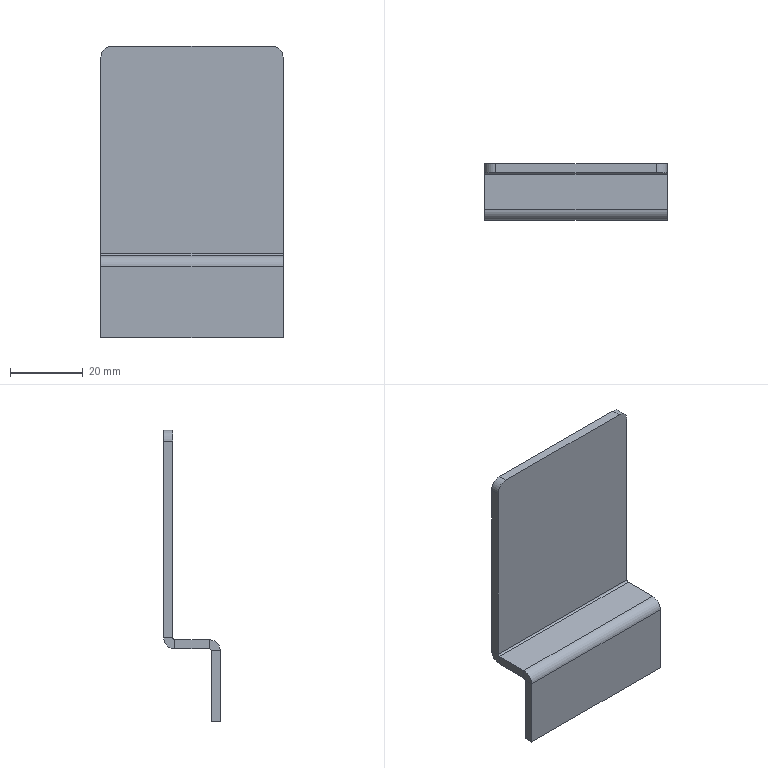Part | SolidWorks | features BaseBody 1 | 1 solid | 24 faces | box 50 x 15.5 x 80 mm | volume 11428 mm3 | plane 18 | cylinder 6 | commonest cylinder face diameters 6 x4 1 x2
STEP:
#1=CARTESIAN_POINT('',(-25.,-6.5,-22.5));
#2=VERTEX_POINT('',#1);
#3=CARTESIAN_POINT('',(25.,-6.5,-22.5));
#4=VERTEX_POINT('',#3);
#5=CARTESIAN_POINT('',(25.,-6.5,-22.5));
#6=DIRECTION('',(1.,0.,0.));
#7=VECTOR('',#6,1000.);
#8=LINE('',#5,#7);
#9=EDGE_CURVE('',#2,#4,#8,.T.);
#10=ORIENTED_EDGE('',*,*,#9,.T.);
#11=CARTESIAN_POINT('',(25.,-9.,-22.5));
#12=VERTEX_POINT('',#11);
#13=CARTESIAN_POINT('',(25.,-9.,-22.5));
#14=DIRECTION('',(0.,1.,0.));
#15=VECTOR('',#14,1000.);
#16=LINE('',#13,#15);
#17=EDGE_CURVE('',#12,#4,#16,.T.);
#18=ORIENTED_EDGE('',*,*,#17,.F.);
#19=CARTESIAN_POINT('',(-25.,-9.,-22.5));
#20=VERTEX_POINT('',#19);
#21=CARTESIAN_POINT('',(25.,-9.,-22.5));
#22=DIRECTION('',(1.,0.,0.));
#23=VECTOR('',#22,1000.);
#24=LINE('',#21,#23);
#25=EDGE_CURVE('',#20,#12,#24,.T.);
#26=ORIENTED_EDGE('',*,*,#25,.F.);
#27=CARTESIAN_POINT('',(-25.,-9.,-22.5));
#28=DIRECTION('',(0.,1.,0.));
#29=VECTOR('',#28,1000.);
#30=LINE('',#27,#29);
#31=EDGE_CURVE('',#20,#2,#30,.T.);
#32=ORIENTED_EDGE('',*,*,#31,.T.);
#33=EDGE_LOOP('',(#10,#18,#26,#32));
#34=FACE_OUTER_BOUND('',#33,.T.);
#35=CARTESIAN_POINT('',(25.,-9.,-22.5));
#36=DIRECTION('',(0.,0.,1.));
#37=DIRECTION('',(0.,-1.,0.));
#38=AXIS2_PLACEMENT_3D('',#35,#36,#37);
#39=PLANE('',#38);
#40=ADVANCED_FACE('',(#34),#39,.F.);
#41=CARTESIAN_POINT('',(-25.,-6.5,-3.));
#42=VERTEX_POINT('',#41);
#43=CARTESIAN_POINT('',(-25.,-6.5,-22.5));
#44=DIRECTION('',(0.,0.,-1.));
#45=VECTOR('',#44,1000.);
#46=LINE('',#43,#45);
#47=EDGE_CURVE('',#42,#2,#46,.T.);
#48=ORIENTED_EDGE('',*,*,#47,.F.);
#49=CARTESIAN_POINT('',(25.,-6.5,-3.));
#50=VERTEX_POINT('',#49);
#51=CARTESIAN_POINT('',(25.,-6.5,-3.));
#52=DIRECTION('',(-1.,0.,0.));
#53=VECTOR('',#52,1000.);
#54=LINE('',#51,#53);
#55=EDGE_CURVE('',#50,#42,#54,.T.);
#56=ORIENTED_EDGE('',*,*,#55,.F.);
#57=CARTESIAN_POINT('',(25.,-6.5,-2.5));
#58=DIRECTION('',(0.,0.,1.));
#59=VECTOR('',#58,1000.);
#60=LINE('',#57,#59);
#61=EDGE_CURVE('',#4,#50,#60,.T.);
#62=ORIENTED_EDGE('',*,*,#61,.F.);
#63=ORIENTED_EDGE('',*,*,#9,.F.);
#64=EDGE_LOOP('',(#48,#56,#62,#63));
#65=FACE_OUTER_BOUND('',#64,.T.);
#66=CARTESIAN_POINT('',(0.,-6.5,0.));
#67=DIRECTION('',(0.,1.,0.));
#68=DIRECTION('',(0.,0.,-1.));
#69=AXIS2_PLACEMENT_3D('',#66,#67,#68);
#70=PLANE('',#69);
#71=ADVANCED_FACE('',(#65),#70,.T.);
#72=CARTESIAN_POINT('',(-25.,-9.,-3.));
#73=VERTEX_POINT('',#72);
#74=CARTESIAN_POINT('',(25.,-9.,-3.));
#75=VERTEX_POINT('',#74);
#76=CARTESIAN_POINT('',(0.,-9.,-3.));
#77=DIRECTION('',(1.,0.,0.));
#78=VECTOR('',#77,1000.);
#79=LINE('',#76,#78);
#80=EDGE_CURVE('',#73,#75,#79,.T.);
#81=ORIENTED_EDGE('',*,*,#80,.F.);
#82=CARTESIAN_POINT('',(-25.,-9.,-22.5));
#83=DIRECTION('',(0.,0.,-1.));
#84=VECTOR('',#83,1000.);
#85=LINE('',#82,#84);
#86=EDGE_CURVE('',#73,#20,#85,.T.);
#87=ORIENTED_EDGE('',*,*,#86,.T.);
#88=ORIENTED_EDGE('',*,*,#25,.T.);
#89=CARTESIAN_POINT('',(25.,-9.,-2.5));
#90=DIRECTION('',(0.,0.,1.));
#91=VECTOR('',#90,1000.);
#92=LINE('',#89,#91);
#93=EDGE_CURVE('',#12,#75,#92,.T.);
#94=ORIENTED_EDGE('',*,*,#93,.T.);
#95=EDGE_LOOP('',(#81,#87,#88,#94));
#96=FACE_OUTER_BOUND('',#95,.T.);
#97=CARTESIAN_POINT('',(0.,-9.,0.));
#98=DIRECTION('',(0.,1.,0.));
#99=DIRECTION('',(0.,0.,-1.));
#100=AXIS2_PLACEMENT_3D('',#97,#98,#99);
#101=PLANE('',#100);
#102=ADVANCED_FACE('',(#96),#101,.F.);
#103=CARTESIAN_POINT('',(25.,-6.5,-3.));
#104=DIRECTION('',(0.,-1.,0.));
#105=VECTOR('',#104,1000.);
#106=LINE('',#103,#105);
#107=EDGE_CURVE('',#50,#75,#106,.T.);
#108=ORIENTED_EDGE('',*,*,#107,.T.);
#109=ORIENTED_EDGE('',*,*,#93,.F.);
#110=ORIENTED_EDGE('',*,*,#17,.T.);
#111=ORIENTED_EDGE('',*,*,#61,.T.);
#112=EDGE_LOOP('',(#108,#109,#110,#111));
#113=FACE_OUTER_BOUND('',#112,.T.);
#114=CARTESIAN_POINT('',(25.,-9.,-2.5));
#115=DIRECTION('',(-1.,0.,0.));
#116=DIRECTION('',(0.,1.,0.));
#117=AXIS2_PLACEMENT_3D('',#114,#115,#116);
#118=PLANE('',#117);
#119=ADVANCED_FACE('',(#113),#118,.F.);
#120=CARTESIAN_POINT('',(-25.,-6.5,-3.));
#121=DIRECTION('',(0.,-1.,0.));
#122=VECTOR('',#121,1000.);
#123=LINE('',#120,#122);
#124=EDGE_CURVE('',#42,#73,#123,.T.);
#125=ORIENTED_EDGE('',*,*,#124,.F.);
#126=ORIENTED_EDGE('',*,*,#47,.T.);
#127=ORIENTED_EDGE('',*,*,#31,.F.);
#128=ORIENTED_EDGE('',*,*,#86,.F.);
#129=EDGE_LOOP('',(#125,#126,#127,#128));
#130=FACE_OUTER_BOUND('',#129,.T.);
#131=CARTESIAN_POINT('',(-25.,-9.,-22.5));
#132=DIRECTION('',(1.,0.,0.));
#133=DIRECTION('',(0.,1.,0.));
#134=AXIS2_PLACEMENT_3D('',#131,#132,#133);
#135=PLANE('',#134);
#136=ADVANCED_FACE('',(#130),#135,.F.);
#137=CARTESIAN_POINT('',(-25.,-6.,-2.5));
#138=VERTEX_POINT('',#137);
#139=CARTESIAN_POINT('',(25.,-6.,-2.5));
#140=VERTEX_POINT('',#139);
#141=CARTESIAN_POINT('',(-25.,-6.,-2.5));
#142=DIRECTION('',(1.,0.,0.));
#143=VECTOR('',#142,1000.);
#144=LINE('',#141,#143);
#145=EDGE_CURVE('',#138,#140,#144,.T.);
#146=ORIENTED_EDGE('',*,*,#145,.T.);
#147=CARTESIAN_POINT('',(25.,-6.,-3.));
#148=DIRECTION('',(1.,0.,0.));
#149=DIRECTION('',(0.,0.,1.));
#150=AXIS2_PLACEMENT_3D('',#147,#148,#149);
#151=CIRCLE('',#150,0.5);
#152=EDGE_CURVE('',#140,#50,#151,.T.);
#153=ORIENTED_EDGE('',*,*,#152,.T.);
#154=ORIENTED_EDGE('',*,*,#55,.T.);
#155=CARTESIAN_POINT('',(-25.,-6.,-3.));
#156=DIRECTION('',(-1.,0.,0.));
#157=DIRECTION('',(0.,0.,1.));
#158=AXIS2_PLACEMENT_3D('',#155,#156,#157);
#159=CIRCLE('',#158,0.5);
#160=EDGE_CURVE('',#42,#138,#159,.T.);
#161=ORIENTED_EDGE('',*,*,#160,.T.);
#162=EDGE_LOOP('',(#146,#153,#154,#161));
#163=FACE_OUTER_BOUND('',#162,.T.);
#164=CARTESIAN_POINT('',(-25.,-6.,-3.));
#165=DIRECTION('',(-1.,0.,0.));
#166=DIRECTION('',(0.,-1.,0.));
#167=AXIS2_PLACEMENT_3D('',#164,#165,#166);
#168=CYLINDRICAL_SURFACE('',#167,0.5);
#169=ADVANCED_FACE('',(#163),#168,.F.);
#170=CARTESIAN_POINT('',(-25.,-6.,0.));
#171=VERTEX_POINT('',#170);
#172=CARTESIAN_POINT('',(25.,-6.,0.));
#173=VERTEX_POINT('',#172);
#174=CARTESIAN_POINT('',(-25.,-6.,0.));
#175=DIRECTION('',(1.,0.,0.));
#176=VECTOR('',#175,1000.);
#177=LINE('',#174,#176);
#178=EDGE_CURVE('',#171,#173,#177,.T.);
#179=ORIENTED_EDGE('',*,*,#178,.F.);
#180=CARTESIAN_POINT('',(-25.,-6.,-3.));
#181=DIRECTION('',(-1.,0.,0.));
#182=DIRECTION('',(0.,0.,1.));
#183=AXIS2_PLACEMENT_3D('',#180,#181,#182);
#184=CIRCLE('',#183,3.);
#185=EDGE_CURVE('',#73,#171,#184,.T.);
#186=ORIENTED_EDGE('',*,*,#185,.F.);
#187=ORIENTED_EDGE('',*,*,#80,.T.);
#188=CARTESIAN_POINT('',(25.,-6.,-3.));
#189=DIRECTION('',(1.,0.,0.));
#190=DIRECTION('',(0.,0.,1.));
#191=AXIS2_PLACEMENT_3D('',#188,#189,#190);
#192=CIRCLE('',#191,3.);
#193=EDGE_CURVE('',#173,#75,#192,.T.);
#194=ORIENTED_EDGE('',*,*,#193,.F.);
#195=EDGE_LOOP('',(#179,#186,#187,#194));
#196=FACE_OUTER_BOUND('',#195,.T.);
#197=CARTESIAN_POINT('',(-25.,-6.,-3.));
#198=DIRECTION('',(-1.,0.,0.));
#199=DIRECTION('',(0.,-1.,0.));
#200=AXIS2_PLACEMENT_3D('',#197,#198,#199);
#201=CYLINDRICAL_SURFACE('',#200,3.);
#202=ADVANCED_FACE('',(#196),#201,.T.);
#203=ORIENTED_EDGE('',*,*,#160,.F.);
#204=ORIENTED_EDGE('',*,*,#124,.T.);
#205=ORIENTED_EDGE('',*,*,#185,.T.);
#206=CARTESIAN_POINT('',(-25.,-6.,-2.5));
#207=DIRECTION('',(0.,0.,1.));
#208=VECTOR('',#207,1000.);
#209=LINE('',#206,#208);
#210=EDGE_CURVE('',#138,#171,#209,.T.);
#211=ORIENTED_EDGE('',*,*,#210,.F.);
#212=EDGE_LOOP('',(#203,#204,#205,#211));
#213=FACE_OUTER_BOUND('',#212,.T.);
#214=CARTESIAN_POINT('',(-25.,-6.,-3.));
#215=DIRECTION('',(1.,0.,0.));
#216=DIRECTION('',(0.,1.,0.));
#217=AXIS2_PLACEMENT_3D('',#214,#215,#216);
#218=PLANE('',#217);
#219=ADVANCED_FACE('',(#213),#218,.F.);
#220=ORIENTED_EDGE('',*,*,#107,.F.);
#221=ORIENTED_EDGE('',*,*,#152,.F.);
#222=CARTESIAN_POINT('',(25.,-6.,-2.5));
#223=DIRECTION('',(0.,0.,1.));
#224=VECTOR('',#223,1000.);
#225=LINE('',#222,#224);
#226=EDGE_CURVE('',#140,#173,#225,.T.);
#227=ORIENTED_EDGE('',*,*,#226,.T.);
#228=ORIENTED_EDGE('',*,*,#193,.T.);
#229=EDGE_LOOP('',(#220,#221,#227,#228));
#230=FACE_OUTER_BOUND('',#229,.T.);
#231=CARTESIAN_POINT('',(25.,-6.,-3.));
#232=DIRECTION('',(1.,0.,0.));
#233=DIRECTION('',(0.,1.,0.));
#234=AXIS2_PLACEMENT_3D('',#231,#232,#233);
#235=PLANE('',#234);
#236=ADVANCED_FACE('',(#230),#235,.T.);
#237=CARTESIAN_POINT('',(-25.,6.5,54.5));
#238=VERTEX_POINT('',#237);
#239=CARTESIAN_POINT('',(-22.,6.5,57.5));
#240=VERTEX_POINT('',#239);
#241=CARTESIAN_POINT('',(-22.,6.5,54.5));
#242=DIRECTION('',(0.,1.,0.));
#243=DIRECTION('',(0.,0.,-1.));
#244=AXIS2_PLACEMENT_3D('',#241,#242,#243);
#245=CIRCLE('',#244,3.);
#246=EDGE_CURVE('',#238,#240,#245,.T.);
#247=ORIENTED_EDGE('',*,*,#246,.F.);
#248=CARTESIAN_POINT('',(-25.,4.,54.5));
#249=VERTEX_POINT('',#248);
#250=CARTESIAN_POINT('',(-25.,6.5,54.5));
#251=DIRECTION('',(0.,1.,0.));
#252=VECTOR('',#251,1000.);
#253=LINE('',#250,#252);
#254=EDGE_CURVE('',#249,#238,#253,.T.);
#255=ORIENTED_EDGE('',*,*,#254,.F.);
#256=CARTESIAN_POINT('',(-22.,4.,57.5));
#257=VERTEX_POINT('',#256);
#258=CARTESIAN_POINT('',(-22.,4.,54.5));
#259=DIRECTION('',(0.,-1.,0.));
#260=DIRECTION('',(0.,0.,-1.));
#261=AXIS2_PLACEMENT_3D('',#258,#259,#260);
#262=CIRCLE('',#261,3.);
#263=EDGE_CURVE('',#257,#249,#262,.T.);
#264=ORIENTED_EDGE('',*,*,#263,.F.);
#265=CARTESIAN_POINT('',(-22.,6.5,57.5));
#266=DIRECTION('',(0.,-1.,0.));
#267=VECTOR('',#266,1000.);
#268=LINE('',#265,#267);
#269=EDGE_CURVE('',#240,#257,#268,.T.);
#270=ORIENTED_EDGE('',*,*,#269,.F.);
#271=EDGE_LOOP('',(#247,#255,#264,#270));
#272=FACE_OUTER_BOUND('',#271,.T.);
#273=CARTESIAN_POINT('',(-22.,6.5,54.5));
#274=DIRECTION('',(0.,-1.,0.));
#275=DIRECTION('',(0.,0.,-1.));
#276=AXIS2_PLACEMENT_3D('',#273,#274,#275);
#277=CYLINDRICAL_SURFACE('',#276,3.);
#278=ADVANCED_FACE('',(#272),#277,.T.);
#279=CARTESIAN_POINT('',(22.,6.5,57.5));
#280=VERTEX_POINT('',#279);
#281=CARTESIAN_POINT('',(25.,6.5,54.5));
#282=VERTEX_POINT('',#281);
#283=CARTESIAN_POINT('',(22.,6.5,54.5));
#284=DIRECTION('',(0.,1.,0.));
#285=DIRECTION('',(0.,0.,-1.));
#286=AXIS2_PLACEMENT_3D('',#283,#284,#285);
#287=CIRCLE('',#286,3.);
#288=EDGE_CURVE('',#280,#282,#287,.T.);
#289=ORIENTED_EDGE('',*,*,#288,.F.);
#290=CARTESIAN_POINT('',(22.,4.,57.5));
#291=VERTEX_POINT('',#290);
#292=CARTESIAN_POINT('',(22.,6.5,57.5));
#293=DIRECTION('',(0.,1.,0.));
#294=VECTOR('',#293,1000.);
#295=LINE('',#292,#294);
#296=EDGE_CURVE('',#291,#280,#295,.T.);
#297=ORIENTED_EDGE('',*,*,#296,.F.);
#298=CARTESIAN_POINT('',(25.,4.,54.5));
#299=VERTEX_POINT('',#298);
#300=CARTESIAN_POINT('',(22.,4.,54.5));
#301=DIRECTION('',(0.,-1.,0.));
#302=DIRECTION('',(0.,0.,-1.));
#303=AXIS2_PLACEMENT_3D('',#300,#301,#302);
#304=CIRCLE('',#303,3.);
#305=EDGE_CURVE('',#299,#291,#304,.T.);
#306=ORIENTED_EDGE('',*,*,#305,.F.);
#307=CARTESIAN_POINT('',(25.,6.5,54.5));
#308=DIRECTION('',(0.,-1.,0.));
#309=VECTOR('',#308,1000.);
#310=LINE('',#307,#309);
#311=EDGE_CURVE('',#282,#299,#310,.T.);
#312=ORIENTED_EDGE('',*,*,#311,.F.);
#313=EDGE_LOOP('',(#289,#297,#306,#312));
#314=FACE_OUTER_BOUND('',#313,.T.);
#315=CARTESIAN_POINT('',(22.,6.5,54.5));
#316=DIRECTION('',(0.,-1.,0.));
#317=DIRECTION('',(0.,0.,-1.));
#318=AXIS2_PLACEMENT_3D('',#315,#316,#317);
#319=CYLINDRICAL_SURFACE('',#318,3.);
#320=ADVANCED_FACE('',(#314),#319,.T.);
#321=CARTESIAN_POINT('',(25.,4.,57.5));
#322=DIRECTION('',(1.,0.,0.));
#323=VECTOR('',#322,1000.);
#324=LINE('',#321,#323);
#325=EDGE_CURVE('',#257,#291,#324,.T.);
#326=ORIENTED_EDGE('',*,*,#325,.T.);
#327=ORIENTED_EDGE('',*,*,#296,.T.);
#328=CARTESIAN_POINT('',(0.,6.5,57.5));
#329=DIRECTION('',(1.,0.,0.));
#330=VECTOR('',#329,1000.);
#331=LINE('',#328,#330);
#332=EDGE_CURVE('',#240,#280,#331,.T.);
#333=ORIENTED_EDGE('',*,*,#332,.F.);
#334=ORIENTED_EDGE('',*,*,#269,.T.);
#335=EDGE_LOOP('',(#326,#327,#333,#334));
#336=FACE_OUTER_BOUND('',#335,.T.);
#337=CARTESIAN_POINT('',(25.,6.5,57.5));
#338=DIRECTION('',(0.,0.,-1.));
#339=DIRECTION('',(0.,-1.,0.));
#340=AXIS2_PLACEMENT_3D('',#337,#338,#339);
#341=PLANE('',#340);
#342=ADVANCED_FACE('',(#336),#341,.F.);
#343=CARTESIAN_POINT('',(25.,4.,0.5));
#344=VERTEX_POINT('',#343);
#345=CARTESIAN_POINT('',(25.,4.,0.));
#346=DIRECTION('',(0.,0.,-1.));
#347=VECTOR('',#346,1000.);
#348=LINE('',#345,#347);
#349=EDGE_CURVE('',#299,#344,#348,.T.);
#350=ORIENTED_EDGE('',*,*,#349,.F.);
#351=ORIENTED_EDGE('',*,*,#305,.T.);
#352=ORIENTED_EDGE('',*,*,#325,.F.);
#353=ORIENTED_EDGE('',*,*,#263,.T.);
#354=CARTESIAN_POINT('',(-25.,4.,0.5));
#355=VERTEX_POINT('',#354);
#356=CARTESIAN_POINT('',(-25.,4.,57.5));
#357=DIRECTION('',(0.,0.,1.));
#358=VECTOR('',#357,1000.);
#359=LINE('',#356,#358);
#360=EDGE_CURVE('',#355,#249,#359,.T.);
#361=ORIENTED_EDGE('',*,*,#360,.F.);
#362=CARTESIAN_POINT('',(25.,4.,0.5));
#363=DIRECTION('',(-1.,0.,0.));
#364=VECTOR('',#363,1000.);
#365=LINE('',#362,#364);
#366=EDGE_CURVE('',#344,#355,#365,.T.);
#367=ORIENTED_EDGE('',*,*,#366,.F.);
#368=EDGE_LOOP('',(#350,#351,#352,#353,#361,#367));
#369=FACE_OUTER_BOUND('',#368,.T.);
#370=CARTESIAN_POINT('',(0.,4.,0.));
#371=DIRECTION('',(0.,-1.,0.));
#372=DIRECTION('',(-1.,0.,0.));
#373=AXIS2_PLACEMENT_3D('',#370,#371,#372);
#374=PLANE('',#373);
#375=ADVANCED_FACE('',(#369),#374,.T.);
#376=ORIENTED_EDGE('',*,*,#332,.T.);
#377=ORIENTED_EDGE('',*,*,#288,.T.);
#378=CARTESIAN_POINT('',(25.,6.5,0.5));
#379=VERTEX_POINT('',#378);
#380=CARTESIAN_POINT('',(25.,6.5,0.));
#381=DIRECTION('',(0.,0.,-1.));
#382=VECTOR('',#381,1000.);
#383=LINE('',#380,#382);
#384=EDGE_CURVE('',#282,#379,#383,.T.);
#385=ORIENTED_EDGE('',*,*,#384,.T.);
#386=CARTESIAN_POINT('',(-25.,6.5,0.5));
#387=VERTEX_POINT('',#386);
#388=CARTESIAN_POINT('',(25.,6.5,0.5));
#389=DIRECTION('',(1.,0.,0.));
#390=VECTOR('',#389,1000.);
#391=LINE('',#388,#390);
#392=EDGE_CURVE('',#387,#379,#391,.T.);
#393=ORIENTED_EDGE('',*,*,#392,.F.);
#394=CARTESIAN_POINT('',(-25.,6.5,0.));
#395=DIRECTION('',(0.,0.,1.));
#396=VECTOR('',#395,1000.);
#397=LINE('',#394,#396);
#398=EDGE_CURVE('',#387,#238,#397,.T.);
#399=ORIENTED_EDGE('',*,*,#398,.T.);
#400=ORIENTED_EDGE('',*,*,#246,.T.);
#401=EDGE_LOOP('',(#376,#377,#385,#393,#399,#400));
#402=FACE_OUTER_BOUND('',#401,.T.);
#403=CARTESIAN_POINT('',(0.,6.5,0.));
#404=DIRECTION('',(0.,-1.,0.));
#405=DIRECTION('',(-1.,0.,0.));
#406=AXIS2_PLACEMENT_3D('',#403,#404,#405);
#407=PLANE('',#406);
#408=ADVANCED_FACE('',(#402),#407,.F.);
#409=ORIENTED_EDGE('',*,*,#360,.T.);
#410=ORIENTED_EDGE('',*,*,#254,.T.);
#411=ORIENTED_EDGE('',*,*,#398,.F.);
#412=CARTESIAN_POINT('',(-25.,4.,0.5));
#413=DIRECTION('',(0.,1.,0.));
#414=VECTOR('',#413,1000.);
#415=LINE('',#412,#414);
#416=EDGE_CURVE('',#355,#387,#415,.T.);
#417=ORIENTED_EDGE('',*,*,#416,.F.);
#418=EDGE_LOOP('',(#409,#410,#411,#417));
#419=FACE_OUTER_BOUND('',#418,.T.);
#420=CARTESIAN_POINT('',(-25.,6.5,57.5));
#421=DIRECTION('',(1.,0.,0.));
#422=DIRECTION('',(0.,1.,0.));
#423=AXIS2_PLACEMENT_3D('',#420,#421,#422);
#424=PLANE('',#423);
#425=ADVANCED_FACE('',(#419),#424,.F.);
#426=ORIENTED_EDGE('',*,*,#384,.F.);
#427=ORIENTED_EDGE('',*,*,#311,.T.);
#428=ORIENTED_EDGE('',*,*,#349,.T.);
#429=CARTESIAN_POINT('',(25.,6.5,0.5));
#430=DIRECTION('',(0.,1.,0.));
#431=VECTOR('',#430,1000.);
#432=LINE('',#429,#431);
#433=EDGE_CURVE('',#344,#379,#432,.T.);
#434=ORIENTED_EDGE('',*,*,#433,.T.);
#435=EDGE_LOOP('',(#426,#427,#428,#434));
#436=FACE_OUTER_BOUND('',#435,.T.);
#437=CARTESIAN_POINT('',(25.,6.5,0.));
#438=DIRECTION('',(-1.,0.,0.));
#439=DIRECTION('',(0.,1.,0.));
#440=AXIS2_PLACEMENT_3D('',#437,#438,#439);
#441=PLANE('',#440);
#442=ADVANCED_FACE('',(#436),#441,.F.);
#443=CARTESIAN_POINT('',(-25.,3.5,0.));
#444=VERTEX_POINT('',#443);
#445=CARTESIAN_POINT('',(25.,3.5,0.));
#446=VERTEX_POINT('',#445);
#447=CARTESIAN_POINT('',(-25.,3.5,0.));
#448=DIRECTION('',(1.,0.,0.));
#449=VECTOR('',#448,1000.);
#450=LINE('',#447,#449);
#451=EDGE_CURVE('',#444,#446,#450,.T.);
#452=ORIENTED_EDGE('',*,*,#451,.T.);
#453=CARTESIAN_POINT('',(25.,3.5,0.5));
#454=DIRECTION('',(1.,0.,0.));
#455=DIRECTION('',(0.,0.,1.));
#456=AXIS2_PLACEMENT_3D('',#453,#454,#455);
#457=CIRCLE('',#456,0.5);
#458=EDGE_CURVE('',#446,#344,#457,.T.);
#459=ORIENTED_EDGE('',*,*,#458,.T.);
#460=ORIENTED_EDGE('',*,*,#366,.T.);
#461=CARTESIAN_POINT('',(-25.,3.5,0.5));
#462=DIRECTION('',(-1.,0.,0.));
#463=DIRECTION('',(0.,0.,1.));
#464=AXIS2_PLACEMENT_3D('',#461,#462,#463);
#465=CIRCLE('',#464,0.5);
#466=EDGE_CURVE('',#355,#444,#465,.T.);
#467=ORIENTED_EDGE('',*,*,#466,.T.);
#468=EDGE_LOOP('',(#452,#459,#460,#467));
#469=FACE_OUTER_BOUND('',#468,.T.);
#470=CARTESIAN_POINT('',(-25.,3.5,0.5));
#471=DIRECTION('',(-1.,0.,0.));
#472=DIRECTION('',(0.,1.,0.));
#473=AXIS2_PLACEMENT_3D('',#470,#471,#472);
#474=CYLINDRICAL_SURFACE('',#473,0.5);
#475=ADVANCED_FACE('',(#469),#474,.F.);
#476=CARTESIAN_POINT('',(-25.,3.5,-2.5));
#477=VERTEX_POINT('',#476);
#478=CARTESIAN_POINT('',(25.,3.5,-2.5));
#479=VERTEX_POINT('',#478);
#480=CARTESIAN_POINT('',(-25.,3.5,-2.5));
#481=DIRECTION('',(1.,0.,0.));
#482=VECTOR('',#481,1000.);
#483=LINE('',#480,#482);
#484=EDGE_CURVE('',#477,#479,#483,.T.);
#485=ORIENTED_EDGE('',*,*,#484,.F.);
#486=CARTESIAN_POINT('',(-25.,3.5,0.5));
#487=DIRECTION('',(-1.,0.,0.));
#488=DIRECTION('',(0.,0.,1.));
#489=AXIS2_PLACEMENT_3D('',#486,#487,#488);
#490=CIRCLE('',#489,3.);
#491=EDGE_CURVE('',#387,#477,#490,.T.);
#492=ORIENTED_EDGE('',*,*,#491,.F.);
#493=ORIENTED_EDGE('',*,*,#392,.T.);
#494=CARTESIAN_POINT('',(25.,3.5,0.5));
#495=DIRECTION('',(1.,0.,0.));
#496=DIRECTION('',(0.,0.,1.));
#497=AXIS2_PLACEMENT_3D('',#494,#495,#496);
#498=CIRCLE('',#497,3.);
#499=EDGE_CURVE('',#479,#379,#498,.T.);
#500=ORIENTED_EDGE('',*,*,#499,.F.);
#501=EDGE_LOOP('',(#485,#492,#493,#500));
#502=FACE_OUTER_BOUND('',#501,.T.);
#503=CARTESIAN_POINT('',(-25.,3.5,0.5));
#504=DIRECTION('',(-1.,0.,0.));
#505=DIRECTION('',(0.,1.,0.));
#506=AXIS2_PLACEMENT_3D('',#503,#504,#505);
#507=CYLINDRICAL_SURFACE('',#506,3.);
#508=ADVANCED_FACE('',(#502),#507,.T.);
#509=ORIENTED_EDGE('',*,*,#466,.F.);
#510=ORIENTED_EDGE('',*,*,#416,.T.);
#511=ORIENTED_EDGE('',*,*,#491,.T.);
#512=CARTESIAN_POINT('',(-25.,3.5,0.));
#513=DIRECTION('',(0.,0.,-1.));
#514=VECTOR('',#513,1000.);
#515=LINE('',#512,#514);
#516=EDGE_CURVE('',#444,#477,#515,.T.);
#517=ORIENTED_EDGE('',*,*,#516,.F.);
#518=EDGE_LOOP('',(#509,#510,#511,#517));
#519=FACE_OUTER_BOUND('',#518,.T.);
#520=CARTESIAN_POINT('',(-25.,3.5,0.5));
#521=DIRECTION('',(1.,0.,0.));
#522=DIRECTION('',(0.,1.,0.));
#523=AXIS2_PLACEMENT_3D('',#520,#521,#522);
#524=PLANE('',#523);
#525=ADVANCED_FACE('',(#519),#524,.F.);
#526=ORIENTED_EDGE('',*,*,#433,.F.);
#527=ORIENTED_EDGE('',*,*,#458,.F.);
#528=CARTESIAN_POINT('',(25.,3.5,0.));
#529=DIRECTION('',(0.,0.,-1.));
#530=VECTOR('',#529,1000.);
#531=LINE('',#528,#530);
#532=EDGE_CURVE('',#446,#479,#531,.T.);
#533=ORIENTED_EDGE('',*,*,#532,.T.);
#534=ORIENTED_EDGE('',*,*,#499,.T.);
#535=EDGE_LOOP('',(#526,#527,#533,#534));
#536=FACE_OUTER_BOUND('',#535,.T.);
#537=CARTESIAN_POINT('',(25.,3.5,0.5));
#538=DIRECTION('',(1.,0.,0.));
#539=DIRECTION('',(0.,1.,0.));
#540=AXIS2_PLACEMENT_3D('',#537,#538,#539);
#541=PLANE('',#540);
#542=ADVANCED_FACE('',(#536),#541,.T.);
#543=ORIENTED_EDGE('',*,*,#226,.F.);
#544=CARTESIAN_POINT('',(25.,6.5,-2.5));
#545=DIRECTION('',(0.,1.,0.));
#546=VECTOR('',#545,1000.);
#547=LINE('',#544,#546);
#548=EDGE_CURVE('',#140,#479,#547,.T.);
#549=ORIENTED_EDGE('',*,*,#548,.T.);
#550=ORIENTED_EDGE('',*,*,#532,.F.);
#551=CARTESIAN_POINT('',(25.,6.5,0.));
#552=DIRECTION('',(0.,1.,0.));
#553=VECTOR('',#552,1000.);
#554=LINE('',#551,#553);
#555=EDGE_CURVE('',#173,#446,#554,.T.);
#556=ORIENTED_EDGE('',*,*,#555,.F.);
#557=EDGE_LOOP('',(#543,#549,#550,#556));
#558=FACE_OUTER_BOUND('',#557,.T.);
#559=CARTESIAN_POINT('',(25.,6.5,-2.5));
#560=DIRECTION('',(1.,0.,0.));
#561=DIRECTION('',(0.,1.,0.));
#562=AXIS2_PLACEMENT_3D('',#559,#560,#561);
#563=PLANE('',#562);
#564=ADVANCED_FACE('',(#558),#563,.T.);
#565=ORIENTED_EDGE('',*,*,#178,.T.);
#566=ORIENTED_EDGE('',*,*,#555,.T.);
#567=ORIENTED_EDGE('',*,*,#451,.F.);
#568=CARTESIAN_POINT('',(-25.,6.5,0.));
#569=DIRECTION('',(0.,-1.,0.));
#570=VECTOR('',#569,1000.);
#571=LINE('',#568,#570);
#572=EDGE_CURVE('',#444,#171,#571,.T.);
#573=ORIENTED_EDGE('',*,*,#572,.T.);
#574=EDGE_LOOP('',(#565,#566,#567,#573));
#575=FACE_OUTER_BOUND('',#574,.T.);
#576=CARTESIAN_POINT('',(0.,0.,0.));
#577=DIRECTION('',(0.,0.,-1.));
#578=DIRECTION('',(0.,-1.,0.));
#579=AXIS2_PLACEMENT_3D('',#576,#577,#578);
#580=PLANE('',#579);
#581=ADVANCED_FACE('',(#575),#580,.F.);
#582=ORIENTED_EDGE('',*,*,#548,.F.);
#583=ORIENTED_EDGE('',*,*,#145,.F.);
#584=CARTESIAN_POINT('',(-25.,6.5,-2.5));
#585=DIRECTION('',(0.,-1.,0.));
#586=VECTOR('',#585,1000.);
#587=LINE('',#584,#586);
#588=EDGE_CURVE('',#477,#138,#587,.T.);
#589=ORIENTED_EDGE('',*,*,#588,.F.);
#590=ORIENTED_EDGE('',*,*,#484,.T.);
#591=EDGE_LOOP('',(#582,#583,#589,#590));
#592=FACE_OUTER_BOUND('',#591,.T.);
#593=CARTESIAN_POINT('',(0.,0.,-2.5));
#594=DIRECTION('',(0.,0.,-1.));
#595=DIRECTION('',(0.,-1.,0.));
#596=AXIS2_PLACEMENT_3D('',#593,#594,#595);
#597=PLANE('',#596);
#598=ADVANCED_FACE('',(#592),#597,.T.);
#599=ORIENTED_EDGE('',*,*,#588,.T.);
#600=ORIENTED_EDGE('',*,*,#210,.T.);
#601=ORIENTED_EDGE('',*,*,#572,.F.);
#602=ORIENTED_EDGE('',*,*,#516,.T.);
#603=EDGE_LOOP('',(#599,#600,#601,#602));
#604=FACE_OUTER_BOUND('',#603,.T.);
#605=CARTESIAN_POINT('',(-25.,6.5,-2.5));
#606=DIRECTION('',(-1.,0.,0.));
#607=DIRECTION('',(0.,0.,1.));
#608=AXIS2_PLACEMENT_3D('',#605,#606,#607);
#609=PLANE('',#608);
#610=ADVANCED_FACE('',(#604),#609,.T.);
#611=CLOSED_SHELL('',(#40,#71,#102,#119,#136,#169,#202,#219,#236,#278,#320,#342,#375,#408,#425,#442,#475,#508,#525,#542,#564,#581,#598,#610));
#612=MANIFOLD_SOLID_BREP('',#611);
#613=CARTESIAN_POINT('',(0.,0.,0.));
#614=DIRECTION('',(0.,0.,1.));
#615=DIRECTION('',(1.,0.,0.));
#616=AXIS2_PLACEMENT_3D('',#613,#614,#615);
#617=(LENGTH_UNIT()NAMED_UNIT(*)SI_UNIT(.MILLI.,.METRE.));
#618=UNCERTAINTY_MEASURE_WITH_UNIT(LENGTH_MEASURE(0.00001),#617,'','');
#619=(NAMED_UNIT(*)PLANE_ANGLE_UNIT()SI_UNIT($,.RADIAN.));
#620=(NAMED_UNIT(*)SI_UNIT($,.STERADIAN.)SOLID_ANGLE_UNIT());
#621=(GEOMETRIC_REPRESENTATION_CONTEXT(3)GLOBAL_UNCERTAINTY_ASSIGNED_CONTEXT((#618))GLOBAL_UNIT_ASSIGNED_CONTEXT((#617,#619,#620))REPRESENTATION_CONTEXT('',''));
#622=ADVANCED_BREP_SHAPE_REPRESENTATION('',(#612,#616),#621);